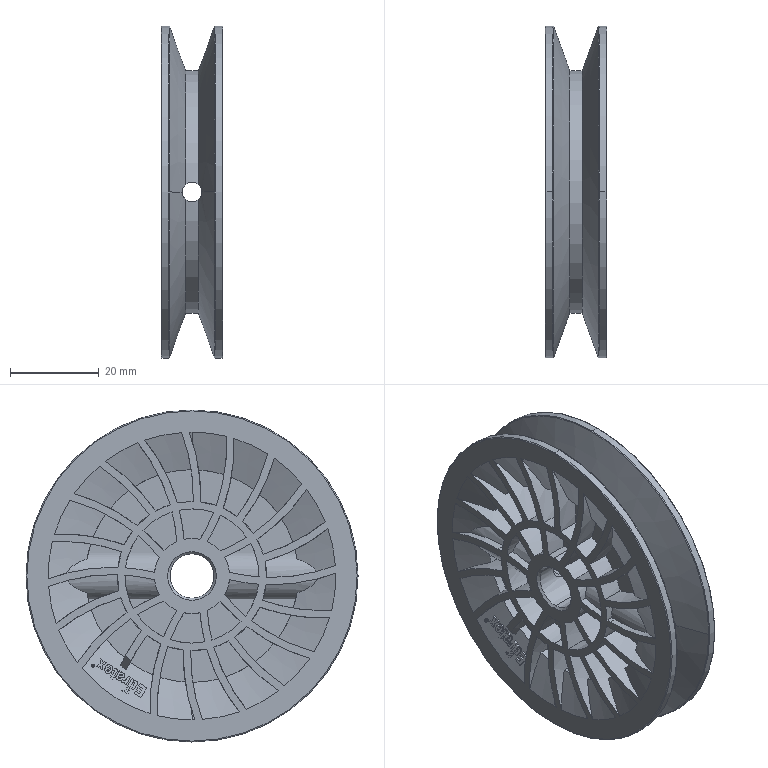Part | STEP file | 101000007597 | 1 solid | 549 faces | box 14 x 75 x 75 mm | volume 33220 mm3 | cylinder 312 | plane 142 | cone 70 | spline 17 | torus 8 | commonest cylinder face diameters 80 x68 83.306 x68 33.7 x44 48 x40 17 x24 30.3 x24